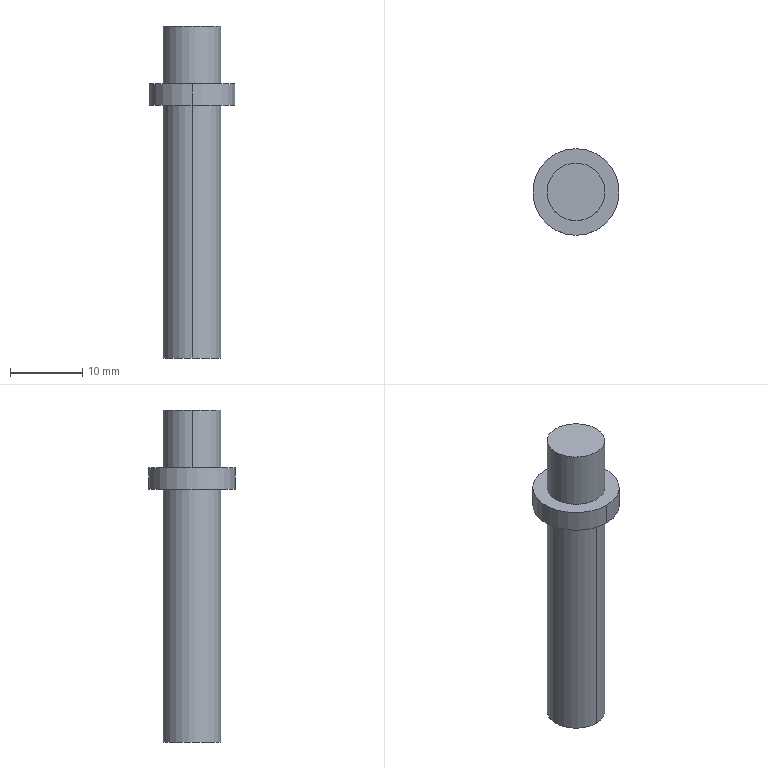Part | SolidWorks | features ICE 3, Extrusion 1 | 1 solid | 10 faces | box 12 x 12 x 46 mm | volume 2501 mm3 | cylinder 6 | plane 4 | commonest cylinder face diameters 8 x4 12 x2
STEP:
#1=CARTESIAN_POINT('',(-145.505,184.569,-46.));
#2=VERTEX_POINT('',#1);
#3=CARTESIAN_POINT('',(-145.505,176.569,-46.));
#4=VERTEX_POINT('',#3);
#5=CARTESIAN_POINT('',(-145.505,180.569,-46.));
#6=DIRECTION('',(0.,0.,-1.));
#7=DIRECTION('',(0.,1.,0.));
#8=AXIS2_PLACEMENT_3D('',#5,#6,#7);
#9=CIRCLE('',#8,4.);
#10=EDGE_CURVE('',#2,#4,#9,.T.);
#11=ORIENTED_EDGE('',*,*,#10,.F.);
#12=CARTESIAN_POINT('',(-145.505,184.569,-11.));
#13=VERTEX_POINT('',#12);
#14=CARTESIAN_POINT('',(-145.505,184.569,-41.));
#15=DIRECTION('',(0.,0.,1.));
#16=VECTOR('',#15,1000.);
#17=LINE('',#14,#16);
#18=EDGE_CURVE('',#2,#13,#17,.T.);
#19=ORIENTED_EDGE('',*,*,#18,.T.);
#20=CARTESIAN_POINT('',(-145.505,176.569,-11.));
#21=VERTEX_POINT('',#20);
#22=CARTESIAN_POINT('',(-145.505,180.569,-11.));
#23=DIRECTION('',(0.,0.,-1.));
#24=DIRECTION('',(0.,1.,0.));
#25=AXIS2_PLACEMENT_3D('',#22,#23,#24);
#26=CIRCLE('',#25,4.);
#27=EDGE_CURVE('',#13,#21,#26,.T.);
#28=ORIENTED_EDGE('',*,*,#27,.T.);
#29=CARTESIAN_POINT('',(-145.505,176.569,-41.));
#30=DIRECTION('',(0.,0.,1.));
#31=VECTOR('',#30,1000.);
#32=LINE('',#29,#31);
#33=EDGE_CURVE('',#4,#21,#32,.T.);
#34=ORIENTED_EDGE('',*,*,#33,.F.);
#35=EDGE_LOOP('',(#11,#19,#28,#34));
#36=FACE_OUTER_BOUND('',#35,.T.);
#37=CARTESIAN_POINT('',(-145.505,180.569,-41.));
#38=DIRECTION('',(0.,0.,1.));
#39=DIRECTION('',(0.,-1.,0.));
#40=AXIS2_PLACEMENT_3D('',#37,#38,#39);
#41=CYLINDRICAL_SURFACE('',#40,4.);
#42=ADVANCED_FACE('',(#36),#41,.T.);
#43=CARTESIAN_POINT('',(-145.505,186.569,-11.));
#44=VERTEX_POINT('',#43);
#45=CARTESIAN_POINT('',(-145.505,174.569,-11.));
#46=VERTEX_POINT('',#45);
#47=CARTESIAN_POINT('',(-145.505,180.569,-11.));
#48=DIRECTION('',(0.,0.,-1.));
#49=DIRECTION('',(0.,1.,0.));
#50=AXIS2_PLACEMENT_3D('',#47,#48,#49);
#51=CIRCLE('',#50,6.);
#52=EDGE_CURVE('',#44,#46,#51,.T.);
#53=ORIENTED_EDGE('',*,*,#52,.F.);
#54=CARTESIAN_POINT('',(-145.505,186.569,-8.));
#55=VERTEX_POINT('',#54);
#56=CARTESIAN_POINT('',(-145.505,186.569,-11.));
#57=DIRECTION('',(0.,0.,1.));
#58=VECTOR('',#57,1000.);
#59=LINE('',#56,#58);
#60=EDGE_CURVE('',#44,#55,#59,.T.);
#61=ORIENTED_EDGE('',*,*,#60,.T.);
#62=CARTESIAN_POINT('',(-145.505,174.569,-8.));
#63=VERTEX_POINT('',#62);
#64=CARTESIAN_POINT('',(-145.505,180.569,-8.));
#65=DIRECTION('',(0.,0.,-1.));
#66=DIRECTION('',(0.,1.,0.));
#67=AXIS2_PLACEMENT_3D('',#64,#65,#66);
#68=CIRCLE('',#67,6.);
#69=EDGE_CURVE('',#55,#63,#68,.T.);
#70=ORIENTED_EDGE('',*,*,#69,.T.);
#71=CARTESIAN_POINT('',(-145.505,174.569,-11.));
#72=DIRECTION('',(0.,0.,1.));
#73=VECTOR('',#72,1000.);
#74=LINE('',#71,#73);
#75=EDGE_CURVE('',#46,#63,#74,.T.);
#76=ORIENTED_EDGE('',*,*,#75,.F.);
#77=EDGE_LOOP('',(#53,#61,#70,#76));
#78=FACE_OUTER_BOUND('',#77,.T.);
#79=CARTESIAN_POINT('',(-145.505,180.569,-11.));
#80=DIRECTION('',(0.,0.,1.));
#81=DIRECTION('',(0.,-1.,0.));
#82=AXIS2_PLACEMENT_3D('',#79,#80,#81);
#83=CYLINDRICAL_SURFACE('',#82,6.);
#84=ADVANCED_FACE('',(#78),#83,.T.);
#85=CARTESIAN_POINT('',(-141.505,180.569,-8.));
#86=VERTEX_POINT('',#85);
#87=CARTESIAN_POINT('',(-149.505,180.569,-8.));
#88=VERTEX_POINT('',#87);
#89=CARTESIAN_POINT('',(-145.505,180.569,-8.));
#90=DIRECTION('',(0.,0.,1.));
#91=DIRECTION('',(0.,1.,0.));
#92=AXIS2_PLACEMENT_3D('',#89,#90,#91);
#93=CIRCLE('',#92,4.);
#94=EDGE_CURVE('',#86,#88,#93,.T.);
#95=ORIENTED_EDGE('',*,*,#94,.T.);
#96=CARTESIAN_POINT('',(-149.505,180.569,0.));
#97=VERTEX_POINT('',#96);
#98=CARTESIAN_POINT('',(-149.505,180.569,-19.314));
#99=DIRECTION('',(0.,0.,1.));
#100=VECTOR('',#99,1000.);
#101=LINE('',#98,#100);
#102=EDGE_CURVE('',#88,#97,#101,.T.);
#103=ORIENTED_EDGE('',*,*,#102,.T.);
#104=CARTESIAN_POINT('',(-141.505,180.569,0.));
#105=VERTEX_POINT('',#104);
#106=CARTESIAN_POINT('',(-145.505,180.569,0.));
#107=DIRECTION('',(0.,0.,1.));
#108=DIRECTION('',(1.,0.,0.));
#109=AXIS2_PLACEMENT_3D('',#106,#107,#108);
#110=CIRCLE('',#109,4.);
#111=EDGE_CURVE('',#105,#97,#110,.T.);
#112=ORIENTED_EDGE('',*,*,#111,.F.);
#113=CARTESIAN_POINT('',(-141.505,180.569,-19.314));
#114=DIRECTION('',(0.,0.,1.));
#115=VECTOR('',#114,1000.);
#116=LINE('',#113,#115);
#117=EDGE_CURVE('',#86,#105,#116,.T.);
#118=ORIENTED_EDGE('',*,*,#117,.F.);
#119=EDGE_LOOP('',(#95,#103,#112,#118));
#120=FACE_OUTER_BOUND('',#119,.T.);
#121=CARTESIAN_POINT('',(-145.505,180.569,-19.314));
#122=DIRECTION('',(0.,0.,1.));
#123=DIRECTION('',(1.,0.,0.));
#124=AXIS2_PLACEMENT_3D('',#121,#122,#123);
#125=CYLINDRICAL_SURFACE('',#124,4.);
#126=ADVANCED_FACE('',(#120),#125,.T.);
#127=ORIENTED_EDGE('',*,*,#111,.T.);
#128=CARTESIAN_POINT('',(-145.505,180.569,0.));
#129=DIRECTION('',(0.,0.,1.));
#130=DIRECTION('',(1.,0.,0.));
#131=AXIS2_PLACEMENT_3D('',#128,#129,#130);
#132=CIRCLE('',#131,4.);
#133=EDGE_CURVE('',#97,#105,#132,.T.);
#134=ORIENTED_EDGE('',*,*,#133,.T.);
#135=EDGE_LOOP('',(#127,#134));
#136=FACE_OUTER_BOUND('',#135,.T.);
#137=CARTESIAN_POINT('',(-145.505,180.569,0.));
#138=DIRECTION('',(0.,0.,1.));
#139=DIRECTION('',(1.,0.,0.));
#140=AXIS2_PLACEMENT_3D('',#137,#138,#139);
#141=PLANE('',#140);
#142=ADVANCED_FACE('',(#136),#141,.T.);
#143=ORIENTED_EDGE('',*,*,#102,.F.);
#144=CARTESIAN_POINT('',(-145.505,180.569,-8.));
#145=DIRECTION('',(0.,0.,1.));
#146=DIRECTION('',(0.,1.,0.));
#147=AXIS2_PLACEMENT_3D('',#144,#145,#146);
#148=CIRCLE('',#147,4.);
#149=EDGE_CURVE('',#88,#86,#148,.T.);
#150=ORIENTED_EDGE('',*,*,#149,.T.);
#151=ORIENTED_EDGE('',*,*,#117,.T.);
#152=ORIENTED_EDGE('',*,*,#133,.F.);
#153=EDGE_LOOP('',(#143,#150,#151,#152));
#154=FACE_OUTER_BOUND('',#153,.T.);
#155=CARTESIAN_POINT('',(-145.505,180.569,-19.314));
#156=DIRECTION('',(0.,0.,1.));
#157=DIRECTION('',(1.,0.,0.));
#158=AXIS2_PLACEMENT_3D('',#155,#156,#157);
#159=CYLINDRICAL_SURFACE('',#158,4.);
#160=ADVANCED_FACE('',(#154),#159,.T.);
#161=ORIENTED_EDGE('',*,*,#60,.F.);
#162=CARTESIAN_POINT('',(-145.505,180.569,-11.));
#163=DIRECTION('',(0.,0.,-1.));
#164=DIRECTION('',(0.,1.,0.));
#165=AXIS2_PLACEMENT_3D('',#162,#163,#164);
#166=CIRCLE('',#165,6.);
#167=EDGE_CURVE('',#46,#44,#166,.T.);
#168=ORIENTED_EDGE('',*,*,#167,.F.);
#169=ORIENTED_EDGE('',*,*,#75,.T.);
#170=CARTESIAN_POINT('',(-145.505,180.569,-8.));
#171=DIRECTION('',(0.,0.,-1.));
#172=DIRECTION('',(0.,1.,0.));
#173=AXIS2_PLACEMENT_3D('',#170,#171,#172);
#174=CIRCLE('',#173,6.);
#175=EDGE_CURVE('',#63,#55,#174,.T.);
#176=ORIENTED_EDGE('',*,*,#175,.T.);
#177=EDGE_LOOP('',(#161,#168,#169,#176));
#178=FACE_OUTER_BOUND('',#177,.T.);
#179=CARTESIAN_POINT('',(-145.505,180.569,-11.));
#180=DIRECTION('',(0.,0.,1.));
#181=DIRECTION('',(0.,-1.,0.));
#182=AXIS2_PLACEMENT_3D('',#179,#180,#181);
#183=CYLINDRICAL_SURFACE('',#182,6.);
#184=ADVANCED_FACE('',(#178),#183,.T.);
#185=CARTESIAN_POINT('',(-145.505,180.569,-11.));
#186=DIRECTION('',(0.,0.,-1.));
#187=DIRECTION('',(0.,1.,0.));
#188=AXIS2_PLACEMENT_3D('',#185,#186,#187);
#189=CIRCLE('',#188,4.);
#190=EDGE_CURVE('',#21,#13,#189,.T.);
#191=ORIENTED_EDGE('',*,*,#190,.F.);
#192=ORIENTED_EDGE('',*,*,#27,.F.);
#193=EDGE_LOOP('',(#191,#192));
#194=FACE_BOUND('',#193,.T.);
#195=ORIENTED_EDGE('',*,*,#167,.T.);
#196=ORIENTED_EDGE('',*,*,#52,.T.);
#197=EDGE_LOOP('',(#195,#196));
#198=FACE_OUTER_BOUND('',#197,.T.);
#199=CARTESIAN_POINT('',(-145.505,180.569,-11.));
#200=DIRECTION('',(0.,0.,-1.));
#201=DIRECTION('',(0.,1.,0.));
#202=AXIS2_PLACEMENT_3D('',#199,#200,#201);
#203=PLANE('',#202);
#204=ADVANCED_FACE('',(#194,#198),#203,.T.);
#205=ORIENTED_EDGE('',*,*,#94,.F.);
#206=ORIENTED_EDGE('',*,*,#149,.F.);
#207=EDGE_LOOP('',(#205,#206));
#208=FACE_BOUND('',#207,.T.);
#209=ORIENTED_EDGE('',*,*,#175,.F.);
#210=ORIENTED_EDGE('',*,*,#69,.F.);
#211=EDGE_LOOP('',(#209,#210));
#212=FACE_OUTER_BOUND('',#211,.T.);
#213=CARTESIAN_POINT('',(-145.505,180.569,-8.));
#214=DIRECTION('',(0.,0.,-1.));
#215=DIRECTION('',(0.,1.,0.));
#216=AXIS2_PLACEMENT_3D('',#213,#214,#215);
#217=PLANE('',#216);
#218=ADVANCED_FACE('',(#208,#212),#217,.F.);
#219=ORIENTED_EDGE('',*,*,#18,.F.);
#220=CARTESIAN_POINT('',(-145.505,180.569,-46.));
#221=DIRECTION('',(0.,0.,-1.));
#222=DIRECTION('',(0.,1.,0.));
#223=AXIS2_PLACEMENT_3D('',#220,#221,#222);
#224=CIRCLE('',#223,4.);
#225=EDGE_CURVE('',#4,#2,#224,.T.);
#226=ORIENTED_EDGE('',*,*,#225,.F.);
#227=ORIENTED_EDGE('',*,*,#33,.T.);
#228=ORIENTED_EDGE('',*,*,#190,.T.);
#229=EDGE_LOOP('',(#219,#226,#227,#228));
#230=FACE_OUTER_BOUND('',#229,.T.);
#231=CARTESIAN_POINT('',(-145.505,180.569,-41.));
#232=DIRECTION('',(0.,0.,1.));
#233=DIRECTION('',(0.,-1.,0.));
#234=AXIS2_PLACEMENT_3D('',#231,#232,#233);
#235=CYLINDRICAL_SURFACE('',#234,4.);
#236=ADVANCED_FACE('',(#230),#235,.T.);
#237=ORIENTED_EDGE('',*,*,#225,.T.);
#238=ORIENTED_EDGE('',*,*,#10,.T.);
#239=EDGE_LOOP('',(#237,#238));
#240=FACE_OUTER_BOUND('',#239,.T.);
#241=CARTESIAN_POINT('',(-145.505,180.569,-46.));
#242=DIRECTION('',(0.,0.,-1.));
#243=DIRECTION('',(0.,1.,0.));
#244=AXIS2_PLACEMENT_3D('',#241,#242,#243);
#245=PLANE('',#244);
#246=ADVANCED_FACE('',(#240),#245,.T.);
#247=CLOSED_SHELL('',(#42,#84,#126,#142,#160,#184,#204,#218,#236,#246));
#248=MANIFOLD_SOLID_BREP('',#247);
#249=CARTESIAN_POINT('',(0.,0.,0.));
#250=DIRECTION('',(0.,0.,1.));
#251=DIRECTION('',(1.,0.,0.));
#252=AXIS2_PLACEMENT_3D('',#249,#250,#251);
#253=(LENGTH_UNIT()NAMED_UNIT(*)SI_UNIT(.MILLI.,.METRE.));
#254=UNCERTAINTY_MEASURE_WITH_UNIT(LENGTH_MEASURE(0.00001),#253,'','');
#255=(NAMED_UNIT(*)PLANE_ANGLE_UNIT()SI_UNIT($,.RADIAN.));
#256=(NAMED_UNIT(*)SI_UNIT($,.STERADIAN.)SOLID_ANGLE_UNIT());
#257=(GEOMETRIC_REPRESENTATION_CONTEXT(3)GLOBAL_UNCERTAINTY_ASSIGNED_CONTEXT((#254))GLOBAL_UNIT_ASSIGNED_CONTEXT((#253,#255,#256))REPRESENTATION_CONTEXT('',''));
#258=ADVANCED_BREP_SHAPE_REPRESENTATION('',(#248,#252),#257);